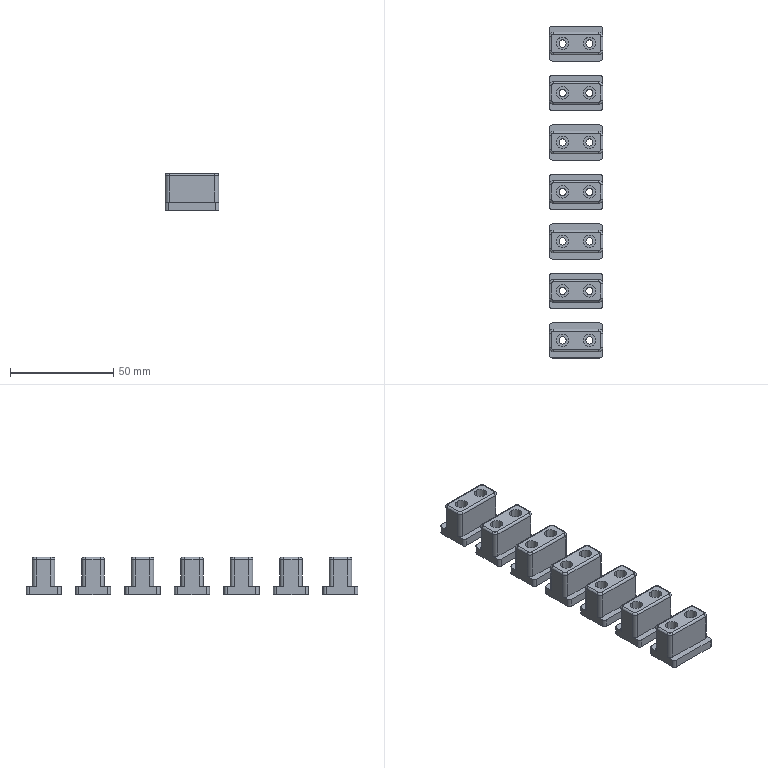Part | 7 solids | 252 faces | box 26 x 161 x 18 mm | volume 35918 mm3 | cylinder 140 | plane 84 | torus 28 | commonest cylinder face diameters 2 x28 3 x28 3.5 x28 4 x28 6 x28